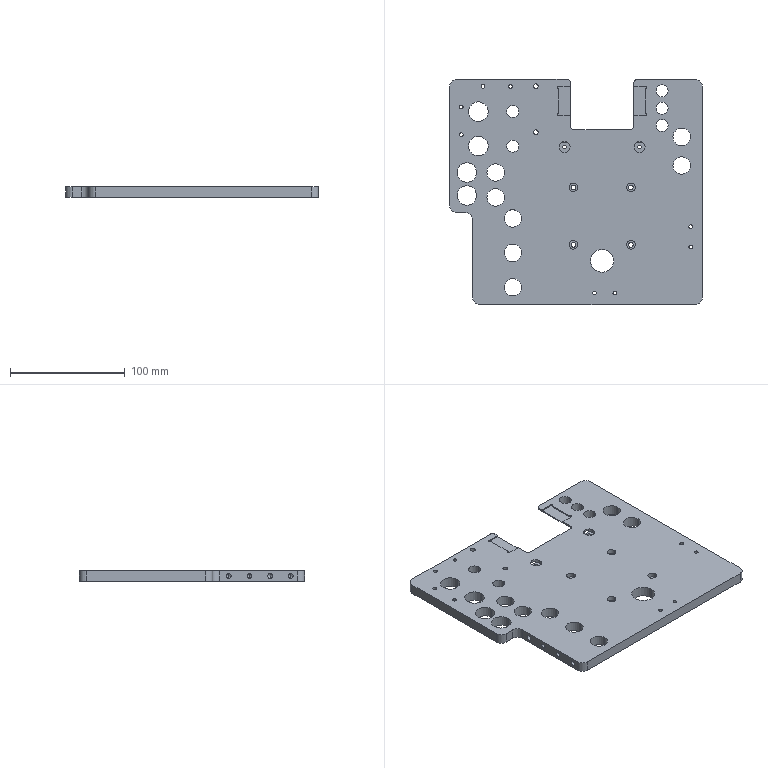Part | 1 solid | 206 faces | box 220 x 196 x 9 mm | volume 302187 mm3 | cylinder 150 | plane 32 | cone 24 | commonest cylinder face diameters 4.2 x60 3.3 x20 15.2 x14 7.5 x12 10.5 x10 12 x10